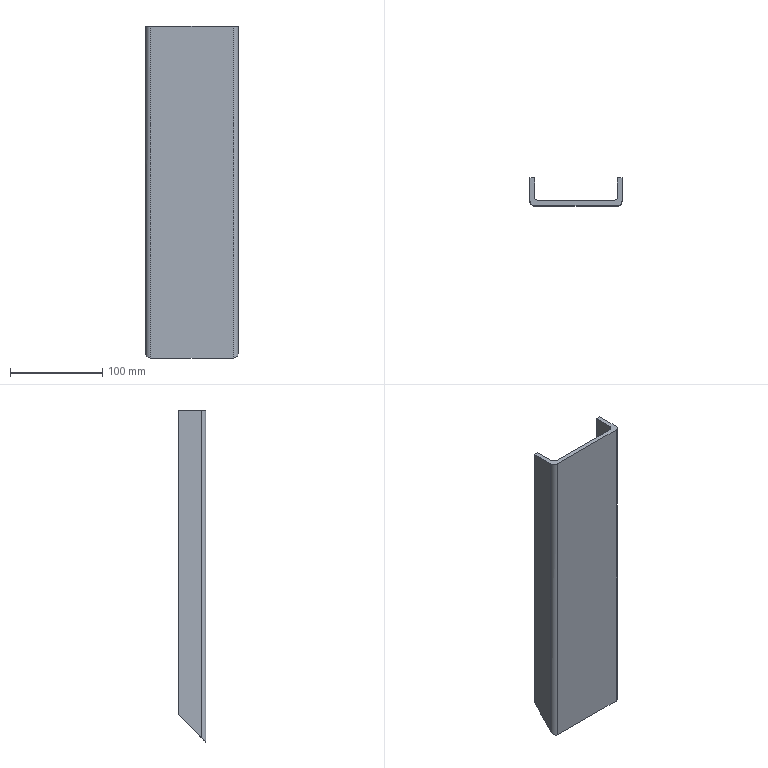Part | SolidWorks | features Extrusion 1, ICE 1 | 1 solid | 14 faces | box 100 x 30 x 360 mm | volume 264321 mm3 | plane 10 | cylinder 4 | commonest cylinder face diameters 10 x4
STEP:
#1=CARTESIAN_POINT('',(100.,30.,30.));
#2=VERTEX_POINT('',#1);
#3=CARTESIAN_POINT('',(95.,30.,30.));
#4=VERTEX_POINT('',#3);
#5=CARTESIAN_POINT('',(100.,30.,30.));
#6=DIRECTION('',(-1.,0.,0.));
#7=VECTOR('',#6,1000.);
#8=LINE('',#5,#7);
#9=EDGE_CURVE('',#2,#4,#8,.T.);
#10=ORIENTED_EDGE('',*,*,#9,.T.);
#11=CARTESIAN_POINT('',(95.,30.,360.));
#12=VERTEX_POINT('',#11);
#13=CARTESIAN_POINT('',(95.,30.,360.));
#14=DIRECTION('',(0.,0.,-1.));
#15=VECTOR('',#14,1000.);
#16=LINE('',#13,#15);
#17=EDGE_CURVE('',#12,#4,#16,.T.);
#18=ORIENTED_EDGE('',*,*,#17,.F.);
#19=CARTESIAN_POINT('',(100.,30.,360.));
#20=VERTEX_POINT('',#19);
#21=CARTESIAN_POINT('',(95.,30.,360.));
#22=DIRECTION('',(-1.,0.,0.));
#23=VECTOR('',#22,1000.);
#24=LINE('',#21,#23);
#25=EDGE_CURVE('',#20,#12,#24,.T.);
#26=ORIENTED_EDGE('',*,*,#25,.F.);
#27=CARTESIAN_POINT('',(100.,30.,360.));
#28=DIRECTION('',(0.,0.,-1.));
#29=VECTOR('',#28,1000.);
#30=LINE('',#27,#29);
#31=EDGE_CURVE('',#20,#2,#30,.T.);
#32=ORIENTED_EDGE('',*,*,#31,.T.);
#33=EDGE_LOOP('',(#10,#18,#26,#32));
#34=FACE_OUTER_BOUND('',#33,.T.);
#35=CARTESIAN_POINT('',(95.,30.,360.));
#36=DIRECTION('',(0.,-1.,0.));
#37=DIRECTION('',(0.,0.,-1.));
#38=AXIS2_PLACEMENT_3D('',#35,#36,#37);
#39=PLANE('',#38);
#40=ADVANCED_FACE('',(#34),#39,.F.);
#41=CARTESIAN_POINT('',(95.,10.,10.));
#42=VERTEX_POINT('',#41);
#43=CARTESIAN_POINT('',(95.,185.,185.));
#44=DIRECTION('',(0.,0.7071,0.7071));
#45=VECTOR('',#44,1000.);
#46=LINE('',#43,#45);
#47=EDGE_CURVE('',#42,#4,#46,.T.);
#48=ORIENTED_EDGE('',*,*,#47,.F.);
#49=CARTESIAN_POINT('',(95.,10.,360.));
#50=VERTEX_POINT('',#49);
#51=CARTESIAN_POINT('',(95.,10.,360.));
#52=DIRECTION('',(0.,0.,-1.));
#53=VECTOR('',#52,1000.);
#54=LINE('',#51,#53);
#55=EDGE_CURVE('',#50,#42,#54,.T.);
#56=ORIENTED_EDGE('',*,*,#55,.F.);
#57=CARTESIAN_POINT('',(95.,10.,360.));
#58=DIRECTION('',(0.,-1.,0.));
#59=VECTOR('',#58,1000.);
#60=LINE('',#57,#59);
#61=EDGE_CURVE('',#12,#50,#60,.T.);
#62=ORIENTED_EDGE('',*,*,#61,.F.);
#63=ORIENTED_EDGE('',*,*,#17,.T.);
#64=EDGE_LOOP('',(#48,#56,#62,#63));
#65=FACE_OUTER_BOUND('',#64,.T.);
#66=CARTESIAN_POINT('',(95.,10.,360.));
#67=DIRECTION('',(1.,0.,0.));
#68=DIRECTION('',(0.,0.,-1.));
#69=AXIS2_PLACEMENT_3D('',#66,#67,#68);
#70=PLANE('',#69);
#71=ADVANCED_FACE('',(#65),#70,.F.);
#72=CARTESIAN_POINT('',(90.,5.,5.));
#73=VERTEX_POINT('',#72);
#74=CARTESIAN_POINT('',(90.,5.,5.));
#75=CARTESIAN_POINT('',(92.929,5.,5.));
#76=CARTESIAN_POINT('',(95.,7.071,7.071));
#77=CARTESIAN_POINT('',(95.,10.,10.));
#78=(BOUNDED_CURVE()B_SPLINE_CURVE(3,(#74,#75,#76,#77),.UNSPECIFIED.,.F.,.F.)B_SPLINE_CURVE_WITH_KNOTS((4,4),(0.,1.571),.UNSPECIFIED.)CURVE()GEOMETRIC_REPRESENTATION_ITEM()RATIONAL_B_SPLINE_CURVE((1.,0.8047,0.8047,1.))REPRESENTATION_ITEM(''));
#79=EDGE_CURVE('',#73,#42,#78,.T.);
#80=ORIENTED_EDGE('',*,*,#79,.F.);
#81=CARTESIAN_POINT('',(90.,5.,360.));
#82=VERTEX_POINT('',#81);
#83=CARTESIAN_POINT('',(90.,5.,360.));
#84=DIRECTION('',(0.,0.,-1.));
#85=VECTOR('',#84,1000.);
#86=LINE('',#83,#85);
#87=EDGE_CURVE('',#82,#73,#86,.T.);
#88=ORIENTED_EDGE('',*,*,#87,.F.);
#89=CARTESIAN_POINT('',(90.,10.,360.));
#90=DIRECTION('',(0.,0.,-1.));
#91=DIRECTION('',(1.,0.,0.));
#92=AXIS2_PLACEMENT_3D('',#89,#90,#91);
#93=CIRCLE('',#92,5.);
#94=EDGE_CURVE('',#50,#82,#93,.T.);
#95=ORIENTED_EDGE('',*,*,#94,.F.);
#96=ORIENTED_EDGE('',*,*,#55,.T.);
#97=EDGE_LOOP('',(#80,#88,#95,#96));
#98=FACE_OUTER_BOUND('',#97,.T.);
#99=CARTESIAN_POINT('',(90.,10.,360.));
#100=DIRECTION('',(0.,0.,-1.));
#101=DIRECTION('',(-1.,0.,0.));
#102=AXIS2_PLACEMENT_3D('',#99,#100,#101);
#103=CYLINDRICAL_SURFACE('',#102,5.);
#104=ADVANCED_FACE('',(#98),#103,.F.);
#105=CARTESIAN_POINT('',(10.,5.,5.));
#106=VERTEX_POINT('',#105);
#107=CARTESIAN_POINT('',(10.,5.,5.));
#108=DIRECTION('',(1.,0.,0.));
#109=VECTOR('',#108,1000.);
#110=LINE('',#107,#109);
#111=EDGE_CURVE('',#106,#73,#110,.T.);
#112=ORIENTED_EDGE('',*,*,#111,.F.);
#113=CARTESIAN_POINT('',(10.,5.,360.));
#114=VERTEX_POINT('',#113);
#115=CARTESIAN_POINT('',(10.,5.,360.));
#116=DIRECTION('',(0.,0.,-1.));
#117=VECTOR('',#116,1000.);
#118=LINE('',#115,#117);
#119=EDGE_CURVE('',#114,#106,#118,.T.);
#120=ORIENTED_EDGE('',*,*,#119,.F.);
#121=CARTESIAN_POINT('',(10.,5.,360.));
#122=DIRECTION('',(-1.,0.,0.));
#123=VECTOR('',#122,1000.);
#124=LINE('',#121,#123);
#125=EDGE_CURVE('',#82,#114,#124,.T.);
#126=ORIENTED_EDGE('',*,*,#125,.F.);
#127=ORIENTED_EDGE('',*,*,#87,.T.);
#128=EDGE_LOOP('',(#112,#120,#126,#127));
#129=FACE_OUTER_BOUND('',#128,.T.);
#130=CARTESIAN_POINT('',(10.,5.,360.));
#131=DIRECTION('',(0.,-1.,0.));
#132=DIRECTION('',(0.,0.,-1.));
#133=AXIS2_PLACEMENT_3D('',#130,#131,#132);
#134=PLANE('',#133);
#135=ADVANCED_FACE('',(#129),#134,.F.);
#136=CARTESIAN_POINT('',(5.,10.,10.));
#137=VERTEX_POINT('',#136);
#138=CARTESIAN_POINT('',(5.,10.,10.));
#139=CARTESIAN_POINT('',(5.,7.071,7.071));
#140=CARTESIAN_POINT('',(7.071,5.,5.));
#141=CARTESIAN_POINT('',(10.,5.,5.));
#142=(BOUNDED_CURVE()B_SPLINE_CURVE(3,(#138,#139,#140,#141),.UNSPECIFIED.,.F.,.F.)B_SPLINE_CURVE_WITH_KNOTS((4,4),(4.712,6.283),.UNSPECIFIED.)CURVE()GEOMETRIC_REPRESENTATION_ITEM()RATIONAL_B_SPLINE_CURVE((1.,0.8047,0.8047,1.))REPRESENTATION_ITEM(''));
#143=EDGE_CURVE('',#137,#106,#142,.T.);
#144=ORIENTED_EDGE('',*,*,#143,.F.);
#145=CARTESIAN_POINT('',(5.,10.,360.));
#146=VERTEX_POINT('',#145);
#147=CARTESIAN_POINT('',(5.,10.,360.));
#148=DIRECTION('',(0.,0.,-1.));
#149=VECTOR('',#148,1000.);
#150=LINE('',#147,#149);
#151=EDGE_CURVE('',#146,#137,#150,.T.);
#152=ORIENTED_EDGE('',*,*,#151,.F.);
#153=CARTESIAN_POINT('',(10.,10.,360.));
#154=DIRECTION('',(0.,0.,-1.));
#155=DIRECTION('',(-1.,0.,0.));
#156=AXIS2_PLACEMENT_3D('',#153,#154,#155);
#157=CIRCLE('',#156,5.);
#158=EDGE_CURVE('',#114,#146,#157,.T.);
#159=ORIENTED_EDGE('',*,*,#158,.F.);
#160=ORIENTED_EDGE('',*,*,#119,.T.);
#161=EDGE_LOOP('',(#144,#152,#159,#160));
#162=FACE_OUTER_BOUND('',#161,.T.);
#163=CARTESIAN_POINT('',(10.,10.,360.));
#164=DIRECTION('',(0.,0.,-1.));
#165=DIRECTION('',(-1.,0.,0.));
#166=AXIS2_PLACEMENT_3D('',#163,#164,#165);
#167=CYLINDRICAL_SURFACE('',#166,5.);
#168=ADVANCED_FACE('',(#162),#167,.F.);
#169=CARTESIAN_POINT('',(5.,30.,30.));
#170=VERTEX_POINT('',#169);
#171=CARTESIAN_POINT('',(5.,185.,185.));
#172=DIRECTION('',(0.,-0.7071,-0.7071));
#173=VECTOR('',#172,1000.);
#174=LINE('',#171,#173);
#175=EDGE_CURVE('',#170,#137,#174,.T.);
#176=ORIENTED_EDGE('',*,*,#175,.F.);
#177=CARTESIAN_POINT('',(5.,30.,360.));
#178=VERTEX_POINT('',#177);
#179=CARTESIAN_POINT('',(5.,30.,360.));
#180=DIRECTION('',(0.,0.,-1.));
#181=VECTOR('',#180,1000.);
#182=LINE('',#179,#181);
#183=EDGE_CURVE('',#178,#170,#182,.T.);
#184=ORIENTED_EDGE('',*,*,#183,.F.);
#185=CARTESIAN_POINT('',(5.,10.,360.));
#186=DIRECTION('',(0.,1.,0.));
#187=VECTOR('',#186,1000.);
#188=LINE('',#185,#187);
#189=EDGE_CURVE('',#146,#178,#188,.T.);
#190=ORIENTED_EDGE('',*,*,#189,.F.);
#191=ORIENTED_EDGE('',*,*,#151,.T.);
#192=EDGE_LOOP('',(#176,#184,#190,#191));
#193=FACE_OUTER_BOUND('',#192,.T.);
#194=CARTESIAN_POINT('',(5.,10.,360.));
#195=DIRECTION('',(-1.,0.,0.));
#196=DIRECTION('',(0.,0.,1.));
#197=AXIS2_PLACEMENT_3D('',#194,#195,#196);
#198=PLANE('',#197);
#199=ADVANCED_FACE('',(#193),#198,.F.);
#200=CARTESIAN_POINT('',(0.,30.,30.));
#201=VERTEX_POINT('',#200);
#202=CARTESIAN_POINT('',(100.,30.,30.));
#203=DIRECTION('',(-1.,0.,0.));
#204=VECTOR('',#203,1000.);
#205=LINE('',#202,#204);
#206=EDGE_CURVE('',#170,#201,#205,.T.);
#207=ORIENTED_EDGE('',*,*,#206,.T.);
#208=CARTESIAN_POINT('',(0.,30.,360.));
#209=VERTEX_POINT('',#208);
#210=CARTESIAN_POINT('',(0.,30.,360.));
#211=DIRECTION('',(0.,0.,-1.));
#212=VECTOR('',#211,1000.);
#213=LINE('',#210,#212);
#214=EDGE_CURVE('',#209,#201,#213,.T.);
#215=ORIENTED_EDGE('',*,*,#214,.F.);
#216=CARTESIAN_POINT('',(0.,30.,360.));
#217=DIRECTION('',(-1.,0.,0.));
#218=VECTOR('',#217,1000.);
#219=LINE('',#216,#218);
#220=EDGE_CURVE('',#178,#209,#219,.T.);
#221=ORIENTED_EDGE('',*,*,#220,.F.);
#222=ORIENTED_EDGE('',*,*,#183,.T.);
#223=EDGE_LOOP('',(#207,#215,#221,#222));
#224=FACE_OUTER_BOUND('',#223,.T.);
#225=CARTESIAN_POINT('',(0.,30.,360.));
#226=DIRECTION('',(0.,-1.,0.));
#227=DIRECTION('',(0.,0.,-1.));
#228=AXIS2_PLACEMENT_3D('',#225,#226,#227);
#229=PLANE('',#228);
#230=ADVANCED_FACE('',(#224),#229,.F.);
#231=CARTESIAN_POINT('',(0.,5.,5.));
#232=VERTEX_POINT('',#231);
#233=CARTESIAN_POINT('',(0.,0.,0.));
#234=DIRECTION('',(0.,-0.7071,-0.7071));
#235=VECTOR('',#234,1000.);
#236=LINE('',#233,#235);
#237=EDGE_CURVE('',#201,#232,#236,.T.);
#238=ORIENTED_EDGE('',*,*,#237,.T.);
#239=CARTESIAN_POINT('',(0.,5.,360.));
#240=VERTEX_POINT('',#239);
#241=CARTESIAN_POINT('',(0.,5.,360.));
#242=DIRECTION('',(0.,0.,-1.));
#243=VECTOR('',#242,1000.);
#244=LINE('',#241,#243);
#245=EDGE_CURVE('',#240,#232,#244,.T.);
#246=ORIENTED_EDGE('',*,*,#245,.F.);
#247=CARTESIAN_POINT('',(0.,5.,360.));
#248=DIRECTION('',(0.,-1.,0.));
#249=VECTOR('',#248,1000.);
#250=LINE('',#247,#249);
#251=EDGE_CURVE('',#209,#240,#250,.T.);
#252=ORIENTED_EDGE('',*,*,#251,.F.);
#253=ORIENTED_EDGE('',*,*,#214,.T.);
#254=EDGE_LOOP('',(#238,#246,#252,#253));
#255=FACE_OUTER_BOUND('',#254,.T.);
#256=CARTESIAN_POINT('',(0.,5.,360.));
#257=DIRECTION('',(1.,0.,0.));
#258=DIRECTION('',(0.,0.,-1.));
#259=AXIS2_PLACEMENT_3D('',#256,#257,#258);
#260=PLANE('',#259);
#261=ADVANCED_FACE('',(#255),#260,.F.);
#262=CARTESIAN_POINT('',(5.,0.,0.));
#263=VERTEX_POINT('',#262);
#264=CARTESIAN_POINT('',(5.,0.,0.));
#265=CARTESIAN_POINT('',(2.071,0.,0.));
#266=CARTESIAN_POINT('',(0.,2.071,2.071));
#267=CARTESIAN_POINT('',(0.,5.,5.));
#268=(BOUNDED_CURVE()B_SPLINE_CURVE(3,(#264,#265,#266,#267),.UNSPECIFIED.,.F.,.T.)B_SPLINE_CURVE_WITH_KNOTS((4,4),(0.,1.571),.UNSPECIFIED.)CURVE()GEOMETRIC_REPRESENTATION_ITEM()RATIONAL_B_SPLINE_CURVE((1.,0.8047,0.8047,1.))REPRESENTATION_ITEM(''));
#269=EDGE_CURVE('',#263,#232,#268,.T.);
#270=ORIENTED_EDGE('',*,*,#269,.F.);
#271=CARTESIAN_POINT('',(5.,0.,360.));
#272=VERTEX_POINT('',#271);
#273=CARTESIAN_POINT('',(5.,0.,360.));
#274=DIRECTION('',(0.,0.,-1.));
#275=VECTOR('',#274,1000.);
#276=LINE('',#273,#275);
#277=EDGE_CURVE('',#272,#263,#276,.T.);
#278=ORIENTED_EDGE('',*,*,#277,.F.);
#279=CARTESIAN_POINT('',(5.,5.,360.));
#280=DIRECTION('',(0.,0.,1.));
#281=DIRECTION('',(-1.,0.,0.));
#282=AXIS2_PLACEMENT_3D('',#279,#280,#281);
#283=CIRCLE('',#282,5.);
#284=EDGE_CURVE('',#240,#272,#283,.T.);
#285=ORIENTED_EDGE('',*,*,#284,.F.);
#286=ORIENTED_EDGE('',*,*,#245,.T.);
#287=EDGE_LOOP('',(#270,#278,#285,#286));
#288=FACE_OUTER_BOUND('',#287,.T.);
#289=CARTESIAN_POINT('',(5.,5.,360.));
#290=DIRECTION('',(0.,0.,-1.));
#291=DIRECTION('',(-1.,0.,0.));
#292=AXIS2_PLACEMENT_3D('',#289,#290,#291);
#293=CYLINDRICAL_SURFACE('',#292,5.);
#294=ADVANCED_FACE('',(#288),#293,.T.);
#295=CARTESIAN_POINT('',(100.,5.,5.));
#296=VERTEX_POINT('',#295);
#297=CARTESIAN_POINT('',(95.,0.,0.));
#298=VERTEX_POINT('',#297);
#299=CARTESIAN_POINT('',(100.,5.,5.));
#300=CARTESIAN_POINT('',(100.,2.071,2.071));
#301=CARTESIAN_POINT('',(97.929,0.,0.));
#302=CARTESIAN_POINT('',(95.,0.,0.));
#303=(BOUNDED_CURVE()B_SPLINE_CURVE(3,(#299,#300,#301,#302),.UNSPECIFIED.,.F.,.F.)B_SPLINE_CURVE_WITH_KNOTS((4,4),(4.712,6.283),.UNSPECIFIED.)CURVE()GEOMETRIC_REPRESENTATION_ITEM()RATIONAL_B_SPLINE_CURVE((1.,0.8047,0.8047,1.))REPRESENTATION_ITEM(''));
#304=EDGE_CURVE('',#296,#298,#303,.T.);
#305=ORIENTED_EDGE('',*,*,#304,.F.);
#306=CARTESIAN_POINT('',(100.,5.,360.));
#307=VERTEX_POINT('',#306);
#308=CARTESIAN_POINT('',(100.,5.,360.));
#309=DIRECTION('',(0.,0.,-1.));
#310=VECTOR('',#309,1000.);
#311=LINE('',#308,#310);
#312=EDGE_CURVE('',#307,#296,#311,.T.);
#313=ORIENTED_EDGE('',*,*,#312,.F.);
#314=CARTESIAN_POINT('',(95.,0.,360.));
#315=VERTEX_POINT('',#314);
#316=CARTESIAN_POINT('',(95.,5.,360.));
#317=DIRECTION('',(0.,0.,1.));
#318=DIRECTION('',(1.,0.,0.));
#319=AXIS2_PLACEMENT_3D('',#316,#317,#318);
#320=CIRCLE('',#319,5.);
#321=EDGE_CURVE('',#315,#307,#320,.T.);
#322=ORIENTED_EDGE('',*,*,#321,.F.);
#323=CARTESIAN_POINT('',(95.,0.,360.));
#324=DIRECTION('',(0.,0.,-1.));
#325=VECTOR('',#324,1000.);
#326=LINE('',#323,#325);
#327=EDGE_CURVE('',#315,#298,#326,.T.);
#328=ORIENTED_EDGE('',*,*,#327,.T.);
#329=EDGE_LOOP('',(#305,#313,#322,#328));
#330=FACE_OUTER_BOUND('',#329,.T.);
#331=CARTESIAN_POINT('',(95.,5.,360.));
#332=DIRECTION('',(0.,0.,-1.));
#333=DIRECTION('',(-1.,0.,0.));
#334=AXIS2_PLACEMENT_3D('',#331,#332,#333);
#335=CYLINDRICAL_SURFACE('',#334,5.);
#336=ADVANCED_FACE('',(#330),#335,.T.);
#337=CARTESIAN_POINT('',(100.,0.,0.));
#338=DIRECTION('',(0.,-0.7071,-0.7071));
#339=VECTOR('',#338,1000.);
#340=LINE('',#337,#339);
#341=EDGE_CURVE('',#2,#296,#340,.T.);
#342=ORIENTED_EDGE('',*,*,#341,.F.);
#343=ORIENTED_EDGE('',*,*,#31,.F.);
#344=CARTESIAN_POINT('',(100.,5.,360.));
#345=DIRECTION('',(0.,1.,0.));
#346=VECTOR('',#345,1000.);
#347=LINE('',#344,#346);
#348=EDGE_CURVE('',#307,#20,#347,.T.);
#349=ORIENTED_EDGE('',*,*,#348,.F.);
#350=ORIENTED_EDGE('',*,*,#312,.T.);
#351=EDGE_LOOP('',(#342,#343,#349,#350));
#352=FACE_OUTER_BOUND('',#351,.T.);
#353=CARTESIAN_POINT('',(100.,5.,360.));
#354=DIRECTION('',(-1.,0.,0.));
#355=DIRECTION('',(0.,0.,1.));
#356=AXIS2_PLACEMENT_3D('',#353,#354,#355);
#357=PLANE('',#356);
#358=ADVANCED_FACE('',(#352),#357,.F.);
#359=CARTESIAN_POINT('',(5.,0.,0.));
#360=DIRECTION('',(1.,0.,0.));
#361=VECTOR('',#360,1000.);
#362=LINE('',#359,#361);
#363=EDGE_CURVE('',#263,#298,#362,.T.);
#364=ORIENTED_EDGE('',*,*,#363,.T.);
#365=ORIENTED_EDGE('',*,*,#327,.F.);
#366=CARTESIAN_POINT('',(5.,0.,360.));
#367=DIRECTION('',(1.,0.,0.));
#368=VECTOR('',#367,1000.);
#369=LINE('',#366,#368);
#370=EDGE_CURVE('',#272,#315,#369,.T.);
#371=ORIENTED_EDGE('',*,*,#370,.F.);
#372=ORIENTED_EDGE('',*,*,#277,.T.);
#373=EDGE_LOOP('',(#364,#365,#371,#372));
#374=FACE_OUTER_BOUND('',#373,.T.);
#375=CARTESIAN_POINT('',(5.,0.,360.));
#376=DIRECTION('',(0.,1.,0.));
#377=DIRECTION('',(0.,0.,1.));
#378=AXIS2_PLACEMENT_3D('',#375,#376,#377);
#379=PLANE('',#378);
#380=ADVANCED_FACE('',(#374),#379,.F.);
#381=ORIENTED_EDGE('',*,*,#25,.T.);
#382=ORIENTED_EDGE('',*,*,#61,.T.);
#383=ORIENTED_EDGE('',*,*,#94,.T.);
#384=ORIENTED_EDGE('',*,*,#125,.T.);
#385=ORIENTED_EDGE('',*,*,#158,.T.);
#386=ORIENTED_EDGE('',*,*,#189,.T.);
#387=ORIENTED_EDGE('',*,*,#220,.T.);
#388=ORIENTED_EDGE('',*,*,#251,.T.);
#389=ORIENTED_EDGE('',*,*,#284,.T.);
#390=ORIENTED_EDGE('',*,*,#370,.T.);
#391=ORIENTED_EDGE('',*,*,#321,.T.);
#392=ORIENTED_EDGE('',*,*,#348,.T.);
#393=EDGE_LOOP('',(#381,#382,#383,#384,#385,#386,#387,#388,#389,#390,#391,#392));
#394=FACE_OUTER_BOUND('',#393,.T.);
#395=CARTESIAN_POINT('',(95.,5.,360.));
#396=DIRECTION('',(0.,0.,1.));
#397=DIRECTION('',(1.,0.,0.));
#398=AXIS2_PLACEMENT_3D('',#395,#396,#397);
#399=PLANE('',#398);
#400=ADVANCED_FACE('',(#394),#399,.T.);
#401=ORIENTED_EDGE('',*,*,#47,.T.);
#402=ORIENTED_EDGE('',*,*,#9,.F.);
#403=ORIENTED_EDGE('',*,*,#341,.T.);
#404=ORIENTED_EDGE('',*,*,#304,.T.);
#405=ORIENTED_EDGE('',*,*,#363,.F.);
#406=ORIENTED_EDGE('',*,*,#269,.T.);
#407=ORIENTED_EDGE('',*,*,#237,.F.);
#408=ORIENTED_EDGE('',*,*,#206,.F.);
#409=ORIENTED_EDGE('',*,*,#175,.T.);
#410=ORIENTED_EDGE('',*,*,#143,.T.);
#411=ORIENTED_EDGE('',*,*,#111,.T.);
#412=ORIENTED_EDGE('',*,*,#79,.T.);
#413=EDGE_LOOP('',(#401,#402,#403,#404,#405,#406,#407,#408,#409,#410,#411,#412));
#414=FACE_OUTER_BOUND('',#413,.T.);
#415=CARTESIAN_POINT('',(100.,0.,0.));
#416=DIRECTION('',(0.,0.7071,-0.7071));
#417=DIRECTION('',(0.,0.7071,0.7071));
#418=AXIS2_PLACEMENT_3D('',#415,#416,#417);
#419=PLANE('',#418);
#420=ADVANCED_FACE('',(#414),#419,.T.);
#421=CLOSED_SHELL('',(#40,#71,#104,#135,#168,#199,#230,#261,#294,#336,#358,#380,#400,#420));
#422=MANIFOLD_SOLID_BREP('',#421);
#423=CARTESIAN_POINT('',(0.,0.,0.));
#424=DIRECTION('',(0.,0.,1.));
#425=DIRECTION('',(1.,0.,0.));
#426=AXIS2_PLACEMENT_3D('',#423,#424,#425);
#427=(LENGTH_UNIT()NAMED_UNIT(*)SI_UNIT(.MILLI.,.METRE.));
#428=UNCERTAINTY_MEASURE_WITH_UNIT(LENGTH_MEASURE(0.00001),#427,'','');
#429=(NAMED_UNIT(*)PLANE_ANGLE_UNIT()SI_UNIT($,.RADIAN.));
#430=(NAMED_UNIT(*)SI_UNIT($,.STERADIAN.)SOLID_ANGLE_UNIT());
#431=(GEOMETRIC_REPRESENTATION_CONTEXT(3)GLOBAL_UNCERTAINTY_ASSIGNED_CONTEXT((#428))GLOBAL_UNIT_ASSIGNED_CONTEXT((#427,#429,#430))REPRESENTATION_CONTEXT('',''));
#432=ADVANCED_BREP_SHAPE_REPRESENTATION('',(#422,#426),#431);